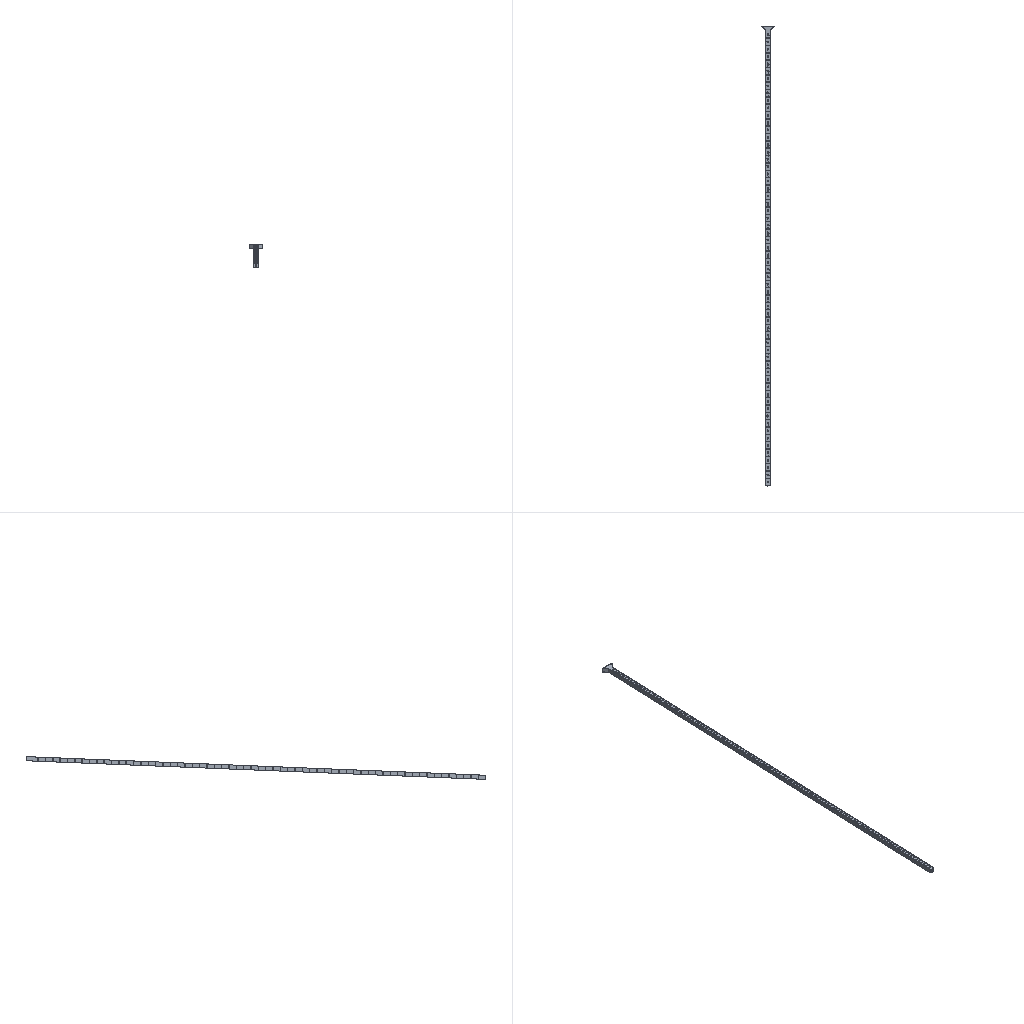Simulation study | ansys fluent
Set-up summary:
category,name,step,type,value,unit,region
solver,ansys_fluent,,Fluent 26.1.0
units,SI m-kg-s (Fluent internal),,stated,boundary values in the units shown in brackets; results in listed units
analysis,deck.cas,,cfd steady,"dimension=3D; solver=3d, dp, pbns, vof, rngke (3d, double precision, pressure-based, VOF, RNG k-epsilon); source_case=.cas"
model,Space,deck.cas,,3D
model,Time,deck.cas,,Steady
model,Viscous,deck.cas,,RNG k-epsilon turbulence model
model,Wall Treatment,deck.cas,,Standard Wall Functions
model,Heat Transfer,deck.cas,,Disabled
model,Multiphase,deck.cas,,Volume of Fluid
mesh,nodes,,,827450
mesh,elements,,,718992
mesh,faces,,,2262926
cell_zone,part_1 (mixture),deck.cas,fluid,material=water-liquid,,zone 3
cell_zone,part_1 (air),deck.cas,fluid,material=air,,zone 3
cell_zone,part_1 (water),deck.cas,fluid,material=water-liquid,,zone 3
material,water-liquid (fluid),,Density,998.2,kg/m^3
material,water-liquid (fluid),,Viscosity,0.001003,kg/(m s)
material,air (fluid),,Density,1.225,kg/m^3
material,air (fluid),,Viscosity,1.7894e-05,kg/(m s)
material,aluminum (solid),,Density,2719,kg/m^3
bc,out1 (mixture),deck.cas,pressure-outlet,Backflow Direction Specification Method=Normal to Boundary,,zone 7
bc,out1 (air),deck.cas,pressure-outlet,,,zone 7
bc,out1 (water),deck.cas,pressure-outlet,,,zone 7
bc,out2 (mixture),deck.cas,pressure-outlet,Backflow Direction Specification Method=Normal to Boundary,,zone 11
bc,out2 (air),deck.cas,pressure-outlet,,,zone 11
bc,out2 (water),deck.cas,pressure-outlet,,,zone 11
bc,int (mixture),deck.cas,velocity-inlet,Velocity Magnitude [m/s]=1,,zone 6
bc,int (air),deck.cas,velocity-inlet,,,zone 6
bc,int (water),deck.cas,velocity-inlet,Volume Fraction=1,,zone 6
bc,wall-part_1 (mixture),deck.cas,wall,Wall Motion=Stationary Wall; Shear Boundary Condition=No Slip,,zone 1
bc,wall-part_1 (air),deck.cas,wall,,,zone 1
bc,wall-part_1 (water),deck.cas,wall,,,zone 1
bc,wall1 (mixture),deck.cas,wall,Wall Motion=Stationary Wall; Shear Boundary Condition=No Slip,,zone 8
bc,wall1 (air),deck.cas,wall,,,zone 8
bc,wall1 (water),deck.cas,wall,,,zone 8
bc,wall2 (mixture),deck.cas,wall,Wall Motion=Stationary Wall; Shear Boundary Condition=No Slip,,zone 9
bc,wall2 (air),deck.cas,wall,,,zone 9
bc,wall2 (water),deck.cas,wall,,,zone 9
bc,wall3 (mixture),deck.cas,wall,Wall Motion=Stationary Wall; Shear Boundary Condition=No Slip,,zone 10
bc,wall3 (air),deck.cas,wall,,,zone 10
bc,wall3 (water),deck.cas,wall,,,zone 10
Results summary:
result,mass flow rate int,deck.cas,,107.806,kg/s
result,mass flow rate out1,deck.cas,,-103.94,kg/s
result,mass flow rate out2,deck.cas,,-1.375,kg/s
result,mass flow rate wall-part_1,deck.cas,,-0,kg/s
result,mass flow rate wall1,deck.cas,,-0,kg/s
result,mass flow rate wall2,deck.cas,,-0,kg/s
result,mass flow rate wall3,deck.cas,,-0,kg/s
result,mass flow rate Net,deck.cas,,2.491,kg/s
result,wall force total wall-part_1,deck.cas,,"(55.038, -241.989, -0.4378)",N
result,wall force pressure wall-part_1,deck.cas,,"(55.039, -241.591, -0.703)",N
result,wall force viscous wall-part_1,deck.cas,,"(-0.001177, -0.3978, 0.2652)",N
result,wall force total wall1,deck.cas,,"(1674.54, -74.551, 0.2373)",N
result,wall force pressure wall1,deck.cas,,"(1674.86, -73.348, 0)",N
result,wall force viscous wall1,deck.cas,,"(-0.3278, -1.203, 0.2373)",N
result,wall force total wall2,deck.cas,,"(-0.007315, 189.374, -4706.02)",N
result,wall force pressure wall2,deck.cas,,"(-0.004698, 190.656, -4705.96)",N
result,wall force viscous wall2,deck.cas,,"(-0.002617, -1.282, -0.05194)",N
result,wall force total wall3,deck.cas,,"(-1729.56, -77.961, 0.2308)",N
result,wall force pressure wall3,deck.cas,,"(-1729.87, -76.725, 0)",N
result,wall force viscous wall3,deck.cas,,"(0.3138, -1.236, 0.2308)",N
result,wall force total Net,deck.cas,,"(0.009222, -205.126, -4705.99)",N
result,wall force pressure Net,deck.cas,,"(0.02702, -201.007, -4706.67)",N
result,wall force viscous Net,deck.cas,,"(-0.01779, -4.119, 0.6813)",N